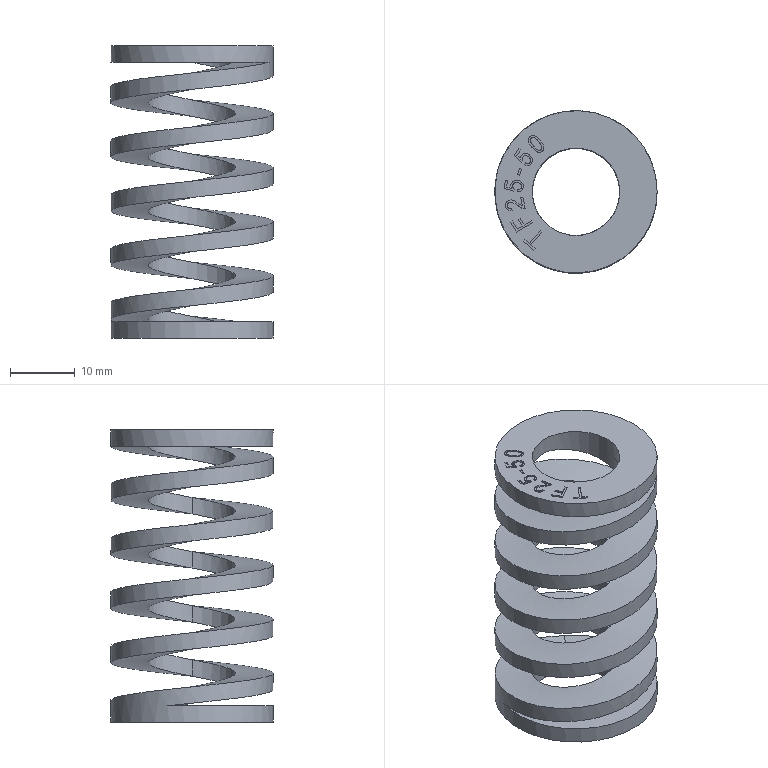Part | STEP file | 1 solid | 99 faces | box 25 x 25 x 45 mm | volume 5947 mm3 | plane 52 | other 35 | cylinder 10 | spline 2 | commonest cylinder face diameters 13.5 x5 25 x5